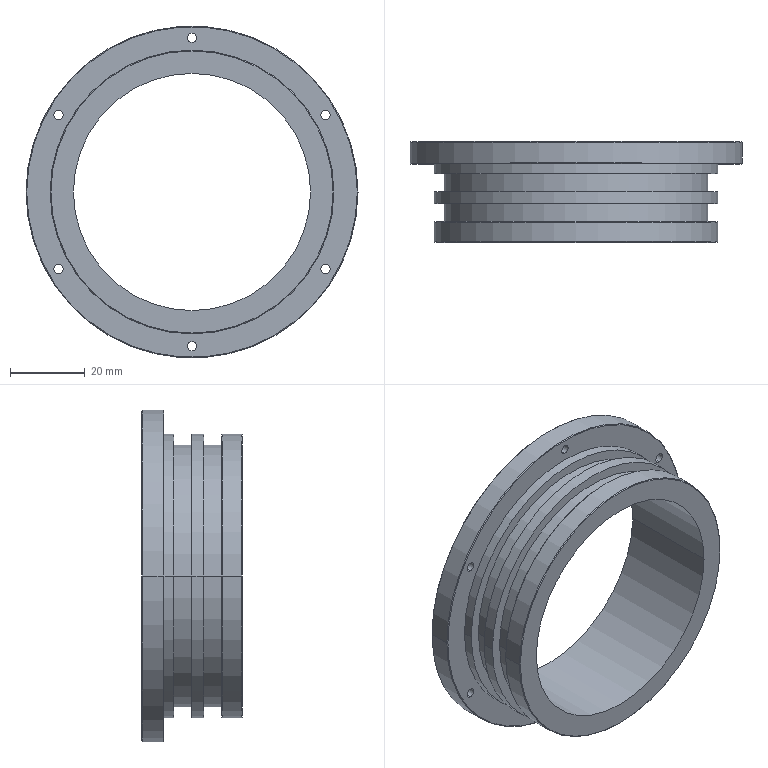Part | SolidWorks | features Chamfer 2, HoleWzd 1, ICE 1, Revolution 1 | 1 solid | 51 faces | box 88.9 x 27 x 88.9 mm | volume 39147 mm3 | cylinder 30 | cone 12 | plane 9 | commonest cylinder face diameters 2.5 x12 75.946 x6 70.561 x4 63.5 x2 70 x2 74.5 x2
STEP:
#1=CARTESIAN_POINT('',(-34.8,27.,0.));
#2=VERTEX_POINT('',#1);
#3=CARTESIAN_POINT('',(34.8,27.,0.));
#4=VERTEX_POINT('',#3);
#5=CARTESIAN_POINT('',(0.,27.,0.));
#6=DIRECTION('',(0.,1.,0.));
#7=DIRECTION('',(-1.,0.,0.));
#8=AXIS2_PLACEMENT_3D('',#5,#6,#7);
#9=CIRCLE('',#8,34.8);
#10=EDGE_CURVE('',#2,#4,#9,.T.);
#11=ORIENTED_EDGE('',*,*,#10,.F.);
#12=CARTESIAN_POINT('',(-35.,26.8,0.));
#13=VERTEX_POINT('',#12);
#14=CARTESIAN_POINT('',(-34.8,27.,0.));
#15=DIRECTION('',(-0.7071,-0.7071,0.));
#16=VECTOR('',#15,1000.);
#17=LINE('',#14,#16);
#18=EDGE_CURVE('',#2,#13,#17,.T.);
#19=ORIENTED_EDGE('',*,*,#18,.T.);
#20=CARTESIAN_POINT('',(35.,26.8,0.));
#21=VERTEX_POINT('',#20);
#22=CARTESIAN_POINT('',(0.,26.8,0.));
#23=DIRECTION('',(0.,-1.,0.));
#24=DIRECTION('',(-1.,0.,0.));
#25=AXIS2_PLACEMENT_3D('',#22,#23,#24);
#26=CIRCLE('',#25,35.);
#27=EDGE_CURVE('',#21,#13,#26,.T.);
#28=ORIENTED_EDGE('',*,*,#27,.F.);
#29=CARTESIAN_POINT('',(34.8,27.,0.));
#30=DIRECTION('',(0.7071,-0.7071,0.));
#31=VECTOR('',#30,1000.);
#32=LINE('',#29,#31);
#33=EDGE_CURVE('',#4,#21,#32,.T.);
#34=ORIENTED_EDGE('',*,*,#33,.F.);
#35=EDGE_LOOP('',(#11,#19,#28,#34));
#36=FACE_OUTER_BOUND('',#35,.T.);
#37=CARTESIAN_POINT('',(0.,27.,0.));
#38=DIRECTION('',(0.,-1.,0.));
#39=DIRECTION('',(1.,0.,0.));
#40=AXIS2_PLACEMENT_3D('',#37,#38,#39);
#41=CONICAL_SURFACE('',#40,34.8,0.7854);
#42=ADVANCED_FACE('',(#36),#41,.T.);
#43=CARTESIAN_POINT('',(37.25,26.8,0.));
#44=VERTEX_POINT('',#43);
#45=CARTESIAN_POINT('',(-37.25,26.8,0.));
#46=VERTEX_POINT('',#45);
#47=CARTESIAN_POINT('',(0.,26.8,0.));
#48=DIRECTION('',(0.,1.,0.));
#49=DIRECTION('',(-1.,0.,0.));
#50=AXIS2_PLACEMENT_3D('',#47,#48,#49);
#51=CIRCLE('',#50,37.25);
#52=EDGE_CURVE('',#44,#46,#51,.T.);
#53=ORIENTED_EDGE('',*,*,#52,.F.);
#54=CARTESIAN_POINT('',(37.45,27.,0.));
#55=VERTEX_POINT('',#54);
#56=CARTESIAN_POINT('',(37.25,26.8,0.));
#57=DIRECTION('',(0.7071,0.7071,0.));
#58=VECTOR('',#57,1000.);
#59=LINE('',#56,#58);
#60=EDGE_CURVE('',#44,#55,#59,.T.);
#61=ORIENTED_EDGE('',*,*,#60,.T.);
#62=CARTESIAN_POINT('',(-37.45,27.,0.));
#63=VERTEX_POINT('',#62);
#64=CARTESIAN_POINT('',(0.,27.,0.));
#65=DIRECTION('',(0.,-1.,0.));
#66=DIRECTION('',(-1.,0.,0.));
#67=AXIS2_PLACEMENT_3D('',#64,#65,#66);
#68=CIRCLE('',#67,37.45);
#69=EDGE_CURVE('',#63,#55,#68,.T.);
#70=ORIENTED_EDGE('',*,*,#69,.F.);
#71=CARTESIAN_POINT('',(-37.25,26.8,0.));
#72=DIRECTION('',(-0.7071,0.7071,0.));
#73=VECTOR('',#72,1000.);
#74=LINE('',#71,#73);
#75=EDGE_CURVE('',#46,#63,#74,.T.);
#76=ORIENTED_EDGE('',*,*,#75,.F.);
#77=EDGE_LOOP('',(#53,#61,#70,#76));
#78=FACE_OUTER_BOUND('',#77,.T.);
#79=CARTESIAN_POINT('',(0.,26.8,0.));
#80=DIRECTION('',(0.,1.,0.));
#81=DIRECTION('',(-1.,0.,0.));
#82=AXIS2_PLACEMENT_3D('',#79,#80,#81);
#83=CONICAL_SURFACE('',#82,37.25,0.7854);
#84=ADVANCED_FACE('',(#78),#83,.F.);
#85=CARTESIAN_POINT('',(-35.,24.,0.));
#86=VERTEX_POINT('',#85);
#87=CARTESIAN_POINT('',(35.,24.,0.));
#88=VERTEX_POINT('',#87);
#89=CARTESIAN_POINT('',(0.,24.,0.));
#90=DIRECTION('',(0.,1.,0.));
#91=DIRECTION('',(-1.,0.,0.));
#92=AXIS2_PLACEMENT_3D('',#89,#90,#91);
#93=CIRCLE('',#92,35.);
#94=EDGE_CURVE('',#86,#88,#93,.T.);
#95=ORIENTED_EDGE('',*,*,#94,.T.);
#96=CARTESIAN_POINT('',(35.,24.,0.));
#97=DIRECTION('',(0.,1.,0.));
#98=VECTOR('',#97,1000.);
#99=LINE('',#96,#98);
#100=EDGE_CURVE('',#88,#21,#99,.T.);
#101=ORIENTED_EDGE('',*,*,#100,.T.);
#102=ORIENTED_EDGE('',*,*,#27,.T.);
#103=CARTESIAN_POINT('',(-35.,24.,0.));
#104=DIRECTION('',(0.,1.,0.));
#105=VECTOR('',#104,1000.);
#106=LINE('',#103,#105);
#107=EDGE_CURVE('',#86,#13,#106,.T.);
#108=ORIENTED_EDGE('',*,*,#107,.F.);
#109=EDGE_LOOP('',(#95,#101,#102,#108));
#110=FACE_OUTER_BOUND('',#109,.T.);
#111=CARTESIAN_POINT('',(0.,24.,0.));
#112=DIRECTION('',(0.,1.,0.));
#113=DIRECTION('',(-1.,0.,0.));
#114=AXIS2_PLACEMENT_3D('',#111,#112,#113);
#115=CYLINDRICAL_SURFACE('',#114,35.);
#116=ADVANCED_FACE('',(#110),#115,.T.);
#117=CARTESIAN_POINT('',(37.25,24.,0.));
#118=VERTEX_POINT('',#117);
#119=CARTESIAN_POINT('',(-37.25,24.,0.));
#120=VERTEX_POINT('',#119);
#121=CARTESIAN_POINT('',(0.,24.,0.));
#122=DIRECTION('',(0.,1.,0.));
#123=DIRECTION('',(-1.,0.,0.));
#124=AXIS2_PLACEMENT_3D('',#121,#122,#123);
#125=CIRCLE('',#124,37.25);
#126=EDGE_CURVE('',#118,#120,#125,.T.);
#127=ORIENTED_EDGE('',*,*,#126,.F.);
#128=CARTESIAN_POINT('',(37.25,24.,0.));
#129=DIRECTION('',(0.,1.,0.));
#130=VECTOR('',#129,1000.);
#131=LINE('',#128,#130);
#132=EDGE_CURVE('',#118,#44,#131,.T.);
#133=ORIENTED_EDGE('',*,*,#132,.T.);
#134=ORIENTED_EDGE('',*,*,#52,.T.);
#135=CARTESIAN_POINT('',(-37.25,24.,0.));
#136=DIRECTION('',(0.,1.,0.));
#137=VECTOR('',#136,1000.);
#138=LINE('',#135,#137);
#139=EDGE_CURVE('',#120,#46,#138,.T.);
#140=ORIENTED_EDGE('',*,*,#139,.F.);
#141=EDGE_LOOP('',(#127,#133,#134,#140));
#142=FACE_OUTER_BOUND('',#141,.T.);
#143=CARTESIAN_POINT('',(0.,24.,0.));
#144=DIRECTION('',(0.,1.,0.));
#145=DIRECTION('',(-1.,0.,0.));
#146=AXIS2_PLACEMENT_3D('',#143,#144,#145);
#147=CYLINDRICAL_SURFACE('',#146,37.25);
#148=ADVANCED_FACE('',(#142),#147,.F.);
#149=CARTESIAN_POINT('',(-35.745,21.,21.888));
#150=VERTEX_POINT('',#149);
#151=CARTESIAN_POINT('',(-35.745,21.,19.388));
#152=VERTEX_POINT('',#151);
#153=CARTESIAN_POINT('',(-35.745,21.,20.638));
#154=DIRECTION('',(0.,-1.,0.));
#155=DIRECTION('',(1.,0.,0.));
#156=AXIS2_PLACEMENT_3D('',#153,#154,#155);
#157=CIRCLE('',#156,1.25);
#158=EDGE_CURVE('',#150,#152,#157,.T.);
#159=ORIENTED_EDGE('',*,*,#158,.T.);
#160=CARTESIAN_POINT('',(-35.745,27.,19.388));
#161=VERTEX_POINT('',#160);
#162=CARTESIAN_POINT('',(-35.745,27.,19.388));
#163=DIRECTION('',(0.,1.,0.));
#164=VECTOR('',#163,1000.);
#165=LINE('',#162,#164);
#166=EDGE_CURVE('',#152,#161,#165,.T.);
#167=ORIENTED_EDGE('',*,*,#166,.T.);
#168=CARTESIAN_POINT('',(-35.745,27.,21.888));
#169=VERTEX_POINT('',#168);
#170=CARTESIAN_POINT('',(-35.745,27.,20.638));
#171=DIRECTION('',(0.,1.,0.));
#172=DIRECTION('',(0.,0.,1.));
#173=AXIS2_PLACEMENT_3D('',#170,#171,#172);
#174=CIRCLE('',#173,1.25);
#175=EDGE_CURVE('',#161,#169,#174,.T.);
#176=ORIENTED_EDGE('',*,*,#175,.T.);
#177=CARTESIAN_POINT('',(-35.745,27.,21.888));
#178=DIRECTION('',(0.,1.,0.));
#179=VECTOR('',#178,1000.);
#180=LINE('',#177,#179);
#181=EDGE_CURVE('',#150,#169,#180,.T.);
#182=ORIENTED_EDGE('',*,*,#181,.F.);
#183=EDGE_LOOP('',(#159,#167,#176,#182));
#184=FACE_OUTER_BOUND('',#183,.T.);
#185=CARTESIAN_POINT('',(-35.745,27.,20.638));
#186=DIRECTION('',(0.,1.,0.));
#187=DIRECTION('',(0.,0.,1.));
#188=AXIS2_PLACEMENT_3D('',#185,#186,#187);
#189=CYLINDRICAL_SURFACE('',#188,1.25);
#190=ADVANCED_FACE('',(#184),#189,.F.);
#191=CARTESIAN_POINT('',(-35.745,21.,-19.388));
#192=VERTEX_POINT('',#191);
#193=CARTESIAN_POINT('',(-35.745,21.,-21.887));
#194=VERTEX_POINT('',#193);
#195=CARTESIAN_POINT('',(-35.745,21.,-20.638));
#196=DIRECTION('',(0.,-1.,0.));
#197=DIRECTION('',(1.,0.,0.));
#198=AXIS2_PLACEMENT_3D('',#195,#196,#197);
#199=CIRCLE('',#198,1.25);
#200=EDGE_CURVE('',#192,#194,#199,.T.);
#201=ORIENTED_EDGE('',*,*,#200,.T.);
#202=CARTESIAN_POINT('',(-35.745,27.,-21.887));
#203=VERTEX_POINT('',#202);
#204=CARTESIAN_POINT('',(-35.745,27.,-21.887));
#205=DIRECTION('',(0.,1.,0.));
#206=VECTOR('',#205,1000.);
#207=LINE('',#204,#206);
#208=EDGE_CURVE('',#194,#203,#207,.T.);
#209=ORIENTED_EDGE('',*,*,#208,.T.);
#210=CARTESIAN_POINT('',(-35.745,27.,-19.388));
#211=VERTEX_POINT('',#210);
#212=CARTESIAN_POINT('',(-35.745,27.,-20.638));
#213=DIRECTION('',(0.,1.,0.));
#214=DIRECTION('',(0.,0.,1.));
#215=AXIS2_PLACEMENT_3D('',#212,#213,#214);
#216=CIRCLE('',#215,1.25);
#217=EDGE_CURVE('',#203,#211,#216,.T.);
#218=ORIENTED_EDGE('',*,*,#217,.T.);
#219=CARTESIAN_POINT('',(-35.745,27.,-19.388));
#220=DIRECTION('',(0.,1.,0.));
#221=VECTOR('',#220,1000.);
#222=LINE('',#219,#221);
#223=EDGE_CURVE('',#192,#211,#222,.T.);
#224=ORIENTED_EDGE('',*,*,#223,.F.);
#225=EDGE_LOOP('',(#201,#209,#218,#224));
#226=FACE_OUTER_BOUND('',#225,.T.);
#227=CARTESIAN_POINT('',(-35.745,27.,-20.638));
#228=DIRECTION('',(0.,1.,0.));
#229=DIRECTION('',(0.,0.,1.));
#230=AXIS2_PLACEMENT_3D('',#227,#228,#229);
#231=CYLINDRICAL_SURFACE('',#230,1.25);
#232=ADVANCED_FACE('',(#226),#231,.F.);
#233=CARTESIAN_POINT('',(0.,21.,-40.025));
#234=VERTEX_POINT('',#233);
#235=CARTESIAN_POINT('',(0.,21.,-42.525));
#236=VERTEX_POINT('',#235);
#237=CARTESIAN_POINT('',(0.,21.,-41.275));
#238=DIRECTION('',(0.,-1.,0.));
#239=DIRECTION('',(1.,0.,0.));
#240=AXIS2_PLACEMENT_3D('',#237,#238,#239);
#241=CIRCLE('',#240,1.25);
#242=EDGE_CURVE('',#234,#236,#241,.T.);
#243=ORIENTED_EDGE('',*,*,#242,.T.);
#244=CARTESIAN_POINT('',(0.,27.,-42.525));
#245=VERTEX_POINT('',#244);
#246=CARTESIAN_POINT('',(0.,27.,-42.525));
#247=DIRECTION('',(0.,1.,0.));
#248=VECTOR('',#247,1000.);
#249=LINE('',#246,#248);
#250=EDGE_CURVE('',#236,#245,#249,.T.);
#251=ORIENTED_EDGE('',*,*,#250,.T.);
#252=CARTESIAN_POINT('',(0.,27.,-40.025));
#253=VERTEX_POINT('',#252);
#254=CARTESIAN_POINT('',(0.,27.,-41.275));
#255=DIRECTION('',(0.,1.,0.));
#256=DIRECTION('',(0.,0.,1.));
#257=AXIS2_PLACEMENT_3D('',#254,#255,#256);
#258=CIRCLE('',#257,1.25);
#259=EDGE_CURVE('',#245,#253,#258,.T.);
#260=ORIENTED_EDGE('',*,*,#259,.T.);
#261=CARTESIAN_POINT('',(0.,27.,-40.025));
#262=DIRECTION('',(0.,1.,0.));
#263=VECTOR('',#262,1000.);
#264=LINE('',#261,#263);
#265=EDGE_CURVE('',#234,#253,#264,.T.);
#266=ORIENTED_EDGE('',*,*,#265,.F.);
#267=EDGE_LOOP('',(#243,#251,#260,#266));
#268=FACE_OUTER_BOUND('',#267,.T.);
#269=CARTESIAN_POINT('',(0.,27.,-41.275));
#270=DIRECTION('',(0.,1.,0.));
#271=DIRECTION('',(0.,0.,1.));
#272=AXIS2_PLACEMENT_3D('',#269,#270,#271);
#273=CYLINDRICAL_SURFACE('',#272,1.25);
#274=ADVANCED_FACE('',(#268),#273,.F.);
#275=CARTESIAN_POINT('',(35.745,21.,-19.388));
#276=VERTEX_POINT('',#275);
#277=CARTESIAN_POINT('',(35.745,21.,-21.888));
#278=VERTEX_POINT('',#277);
#279=CARTESIAN_POINT('',(35.745,21.,-20.638));
#280=DIRECTION('',(0.,-1.,0.));
#281=DIRECTION('',(1.,0.,0.));
#282=AXIS2_PLACEMENT_3D('',#279,#280,#281);
#283=CIRCLE('',#282,1.25);
#284=EDGE_CURVE('',#276,#278,#283,.T.);
#285=ORIENTED_EDGE('',*,*,#284,.T.);
#286=CARTESIAN_POINT('',(35.745,27.,-21.888));
#287=VERTEX_POINT('',#286);
#288=CARTESIAN_POINT('',(35.745,27.,-21.888));
#289=DIRECTION('',(0.,1.,0.));
#290=VECTOR('',#289,1000.);
#291=LINE('',#288,#290);
#292=EDGE_CURVE('',#278,#287,#291,.T.);
#293=ORIENTED_EDGE('',*,*,#292,.T.);
#294=CARTESIAN_POINT('',(35.745,27.,-19.388));
#295=VERTEX_POINT('',#294);
#296=CARTESIAN_POINT('',(35.745,27.,-20.638));
#297=DIRECTION('',(0.,1.,0.));
#298=DIRECTION('',(0.,0.,1.));
#299=AXIS2_PLACEMENT_3D('',#296,#297,#298);
#300=CIRCLE('',#299,1.25);
#301=EDGE_CURVE('',#287,#295,#300,.T.);
#302=ORIENTED_EDGE('',*,*,#301,.T.);
#303=CARTESIAN_POINT('',(35.745,27.,-19.388));
#304=DIRECTION('',(0.,1.,0.));
#305=VECTOR('',#304,1000.);
#306=LINE('',#303,#305);
#307=EDGE_CURVE('',#276,#295,#306,.T.);
#308=ORIENTED_EDGE('',*,*,#307,.F.);
#309=EDGE_LOOP('',(#285,#293,#302,#308));
#310=FACE_OUTER_BOUND('',#309,.T.);
#311=CARTESIAN_POINT('',(35.745,27.,-20.638));
#312=DIRECTION('',(0.,1.,0.));
#313=DIRECTION('',(0.,0.,1.));
#314=AXIS2_PLACEMENT_3D('',#311,#312,#313);
#315=CYLINDRICAL_SURFACE('',#314,1.25);
#316=ADVANCED_FACE('',(#310),#315,.F.);
#317=CARTESIAN_POINT('',(35.745,21.,21.887));
#318=VERTEX_POINT('',#317);
#319=CARTESIAN_POINT('',(35.745,21.,19.388));
#320=VERTEX_POINT('',#319);
#321=CARTESIAN_POINT('',(35.745,21.,20.637));
#322=DIRECTION('',(0.,-1.,0.));
#323=DIRECTION('',(1.,0.,0.));
#324=AXIS2_PLACEMENT_3D('',#321,#322,#323);
#325=CIRCLE('',#324,1.25);
#326=EDGE_CURVE('',#318,#320,#325,.T.);
#327=ORIENTED_EDGE('',*,*,#326,.T.);
#328=CARTESIAN_POINT('',(35.745,27.,19.388));
#329=VERTEX_POINT('',#328);
#330=CARTESIAN_POINT('',(35.745,27.,19.388));
#331=DIRECTION('',(0.,1.,0.));
#332=VECTOR('',#331,1000.);
#333=LINE('',#330,#332);
#334=EDGE_CURVE('',#320,#329,#333,.T.);
#335=ORIENTED_EDGE('',*,*,#334,.T.);
#336=CARTESIAN_POINT('',(35.745,27.,21.887));
#337=VERTEX_POINT('',#336);
#338=CARTESIAN_POINT('',(35.745,27.,20.637));
#339=DIRECTION('',(0.,1.,0.));
#340=DIRECTION('',(0.,0.,1.));
#341=AXIS2_PLACEMENT_3D('',#338,#339,#340);
#342=CIRCLE('',#341,1.25);
#343=EDGE_CURVE('',#329,#337,#342,.T.);
#344=ORIENTED_EDGE('',*,*,#343,.T.);
#345=CARTESIAN_POINT('',(35.745,27.,21.887));
#346=DIRECTION('',(0.,1.,0.));
#347=VECTOR('',#346,1000.);
#348=LINE('',#345,#347);
#349=EDGE_CURVE('',#318,#337,#348,.T.);
#350=ORIENTED_EDGE('',*,*,#349,.F.);
#351=EDGE_LOOP('',(#327,#335,#344,#350));
#352=FACE_OUTER_BOUND('',#351,.T.);
#353=CARTESIAN_POINT('',(35.745,27.,20.637));
#354=DIRECTION('',(0.,1.,0.));
#355=DIRECTION('',(0.,0.,1.));
#356=AXIS2_PLACEMENT_3D('',#353,#354,#355);
#357=CYLINDRICAL_SURFACE('',#356,1.25);
#358=ADVANCED_FACE('',(#352),#357,.F.);
#359=CARTESIAN_POINT('',(0.,21.,42.525));
#360=VERTEX_POINT('',#359);
#361=CARTESIAN_POINT('',(0.,21.,40.025));
#362=VERTEX_POINT('',#361);
#363=CARTESIAN_POINT('',(0.,21.,41.275));
#364=DIRECTION('',(0.,-1.,0.));
#365=DIRECTION('',(1.,0.,0.));
#366=AXIS2_PLACEMENT_3D('',#363,#364,#365);
#367=CIRCLE('',#366,1.25);
#368=EDGE_CURVE('',#360,#362,#367,.T.);
#369=ORIENTED_EDGE('',*,*,#368,.T.);
#370=CARTESIAN_POINT('',(0.,27.,40.025));
#371=VERTEX_POINT('',#370);
#372=CARTESIAN_POINT('',(0.,27.,40.025));
#373=DIRECTION('',(0.,1.,0.));
#374=VECTOR('',#373,1000.);
#375=LINE('',#372,#374);
#376=EDGE_CURVE('',#362,#371,#375,.T.);
#377=ORIENTED_EDGE('',*,*,#376,.T.);
#378=CARTESIAN_POINT('',(0.,27.,42.525));
#379=VERTEX_POINT('',#378);
#380=CARTESIAN_POINT('',(0.,27.,41.275));
#381=DIRECTION('',(0.,1.,0.));
#382=DIRECTION('',(0.,0.,1.));
#383=AXIS2_PLACEMENT_3D('',#380,#381,#382);
#384=CIRCLE('',#383,1.25);
#385=EDGE_CURVE('',#371,#379,#384,.T.);
#386=ORIENTED_EDGE('',*,*,#385,.T.);
#387=CARTESIAN_POINT('',(0.,27.,42.525));
#388=DIRECTION('',(0.,1.,0.));
#389=VECTOR('',#388,1000.);
#390=LINE('',#387,#389);
#391=EDGE_CURVE('',#360,#379,#390,.T.);
#392=ORIENTED_EDGE('',*,*,#391,.F.);
#393=EDGE_LOOP('',(#369,#377,#386,#392));
#394=FACE_OUTER_BOUND('',#393,.T.);
#395=CARTESIAN_POINT('',(0.,27.,41.275));
#396=DIRECTION('',(0.,1.,0.));
#397=DIRECTION('',(0.,0.,1.));
#398=AXIS2_PLACEMENT_3D('',#395,#396,#397);
#399=CYLINDRICAL_SURFACE('',#398,1.25);
#400=ADVANCED_FACE('',(#394),#399,.F.);
#401=CARTESIAN_POINT('',(44.25,21.,0.));
#402=VERTEX_POINT('',#401);
#403=CARTESIAN_POINT('',(-44.25,21.,0.));
#404=VERTEX_POINT('',#403);
#405=CARTESIAN_POINT('',(0.,21.,0.));
#406=DIRECTION('',(0.,-1.,0.));
#407=DIRECTION('',(1.,0.,0.));
#408=AXIS2_PLACEMENT_3D('',#405,#406,#407);
#409=CIRCLE('',#408,44.25);
#410=EDGE_CURVE('',#402,#404,#409,.T.);
#411=ORIENTED_EDGE('',*,*,#410,.F.);
#412=CARTESIAN_POINT('',(44.45,21.2,0.));
#413=VERTEX_POINT('',#412);
#414=CARTESIAN_POINT('',(44.45,21.2,0.));
#415=DIRECTION('',(0.7071,0.7071,0.));
#416=VECTOR('',#415,1000.);
#417=LINE('',#414,#416);
#418=EDGE_CURVE('',#402,#413,#417,.T.);
#419=ORIENTED_EDGE('',*,*,#418,.T.);
#420=CARTESIAN_POINT('',(-44.45,21.2,0.));
#421=VERTEX_POINT('',#420);
#422=CARTESIAN_POINT('',(0.,21.2,0.));
#423=DIRECTION('',(0.,1.,0.));
#424=DIRECTION('',(1.,0.,0.));
#425=AXIS2_PLACEMENT_3D('',#422,#423,#424);
#426=CIRCLE('',#425,44.45);
#427=EDGE_CURVE('',#421,#413,#426,.T.);
#428=ORIENTED_EDGE('',*,*,#427,.F.);
#429=CARTESIAN_POINT('',(-44.45,21.2,0.));
#430=DIRECTION('',(-0.7071,0.7071,0.));
#431=VECTOR('',#430,1000.);
#432=LINE('',#429,#431);
#433=EDGE_CURVE('',#404,#421,#432,.T.);
#434=ORIENTED_EDGE('',*,*,#433,.F.);
#435=EDGE_LOOP('',(#411,#419,#428,#434));
#436=FACE_OUTER_BOUND('',#435,.T.);
#437=CARTESIAN_POINT('',(0.,21.2,0.));
#438=DIRECTION('',(0.,1.,0.));
#439=DIRECTION('',(-1.,0.,0.));
#440=AXIS2_PLACEMENT_3D('',#437,#438,#439);
#441=CONICAL_SURFACE('',#440,44.45,0.7854);
#442=ADVANCED_FACE('',(#436),#441,.T.);
#443=CARTESIAN_POINT('',(-44.25,27.,0.));
#444=VERTEX_POINT('',#443);
#445=CARTESIAN_POINT('',(44.25,27.,0.));
#446=VERTEX_POINT('',#445);
#447=CARTESIAN_POINT('',(0.,27.,0.));
#448=DIRECTION('',(0.,1.,0.));
#449=DIRECTION('',(-1.,0.,0.));
#450=AXIS2_PLACEMENT_3D('',#447,#448,#449);
#451=CIRCLE('',#450,44.25);
#452=EDGE_CURVE('',#444,#446,#451,.T.);
#453=ORIENTED_EDGE('',*,*,#452,.F.);
#454=CARTESIAN_POINT('',(-44.45,26.8,0.));
#455=VERTEX_POINT('',#454);
#456=CARTESIAN_POINT('',(-44.25,27.,0.));
#457=DIRECTION('',(-0.7071,-0.7071,0.));
#458=VECTOR('',#457,1000.);
#459=LINE('',#456,#458);
#460=EDGE_CURVE('',#444,#455,#459,.T.);
#461=ORIENTED_EDGE('',*,*,#460,.T.);
#462=CARTESIAN_POINT('',(44.45,26.8,0.));
#463=VERTEX_POINT('',#462);
#464=CARTESIAN_POINT('',(0.,26.8,0.));
#465=DIRECTION('',(0.,-1.,0.));
#466=DIRECTION('',(-1.,0.,0.));
#467=AXIS2_PLACEMENT_3D('',#464,#465,#466);
#468=CIRCLE('',#467,44.45);
#469=EDGE_CURVE('',#463,#455,#468,.T.);
#470=ORIENTED_EDGE('',*,*,#469,.F.);
#471=CARTESIAN_POINT('',(44.25,27.,0.));
#472=DIRECTION('',(0.7071,-0.7071,0.));
#473=VECTOR('',#472,1000.);
#474=LINE('',#471,#473);
#475=EDGE_CURVE('',#446,#463,#474,.T.);
#476=ORIENTED_EDGE('',*,*,#475,.F.);
#477=EDGE_LOOP('',(#453,#461,#470,#476));
#478=FACE_OUTER_BOUND('',#477,.T.);
#479=CARTESIAN_POINT('',(0.,27.,0.));
#480=DIRECTION('',(0.,-1.,0.));
#481=DIRECTION('',(1.,0.,0.));
#482=AXIS2_PLACEMENT_3D('',#479,#480,#481);
#483=CONICAL_SURFACE('',#482,44.25,0.7854);
#484=ADVANCED_FACE('',(#478),#483,.T.);
#485=CARTESIAN_POINT('',(37.773,0.,0.));
#486=VERTEX_POINT('',#485);
#487=CARTESIAN_POINT('',(-37.773,0.,0.));
#488=VERTEX_POINT('',#487);
#489=CARTESIAN_POINT('',(0.,0.,0.));
#490=DIRECTION('',(0.,-1.,0.));
#491=DIRECTION('',(1.,0.,0.));
#492=AXIS2_PLACEMENT_3D('',#489,#490,#491);
#493=CIRCLE('',#492,37.773);
#494=EDGE_CURVE('',#486,#488,#493,.T.);
#495=ORIENTED_EDGE('',*,*,#494,.F.);
#496=CARTESIAN_POINT('',(37.973,0.2,0.));
#497=VERTEX_POINT('',#496);
#498=CARTESIAN_POINT('',(37.973,0.2,0.));
#499=DIRECTION('',(0.7071,0.7071,0.));
#500=VECTOR('',#499,1000.);
#501=LINE('',#498,#500);
#502=EDGE_CURVE('',#486,#497,#501,.T.);
#503=ORIENTED_EDGE('',*,*,#502,.T.);
#504=CARTESIAN_POINT('',(-37.973,0.2,0.));
#505=VERTEX_POINT('',#504);
#506=CARTESIAN_POINT('',(0.,0.2,0.));
#507=DIRECTION('',(0.,1.,0.));
#508=DIRECTION('',(1.,0.,0.));
#509=AXIS2_PLACEMENT_3D('',#506,#507,#508);
#510=CIRCLE('',#509,37.973);
#511=EDGE_CURVE('',#505,#497,#510,.T.);
#512=ORIENTED_EDGE('',*,*,#511,.F.);
#513=CARTESIAN_POINT('',(-37.973,0.2,0.));
#514=DIRECTION('',(-0.7071,0.7071,0.));
#515=VECTOR('',#514,1000.);
#516=LINE('',#513,#515);
#517=EDGE_CURVE('',#488,#505,#516,.T.);
#518=ORIENTED_EDGE('',*,*,#517,.F.);
#519=EDGE_LOOP('',(#495,#503,#512,#518));
#520=FACE_OUTER_BOUND('',#519,.T.);
#521=CARTESIAN_POINT('',(0.,0.2,0.));
#522=DIRECTION('',(0.,1.,0.));
#523=DIRECTION('',(-1.,0.,0.));
#524=AXIS2_PLACEMENT_3D('',#521,#522,#523);
#525=CONICAL_SURFACE('',#524,37.973,0.7854);
#526=ADVANCED_FACE('',(#520),#525,.T.);
#527=CARTESIAN_POINT('',(-37.773,5.587,0.));
#528=VERTEX_POINT('',#527);
#529=CARTESIAN_POINT('',(37.773,5.587,0.));
#530=VERTEX_POINT('',#529);
#531=CARTESIAN_POINT('',(0.,5.587,0.));
#532=DIRECTION('',(0.,1.,0.));
#533=DIRECTION('',(-1.,0.,0.));
#534=AXIS2_PLACEMENT_3D('',#531,#532,#533);
#535=CIRCLE('',#534,37.773);
#536=EDGE_CURVE('',#528,#530,#535,.T.);
#537=ORIENTED_EDGE('',*,*,#536,.F.);
#538=CARTESIAN_POINT('',(-37.973,5.387,0.));
#539=VERTEX_POINT('',#538);
#540=CARTESIAN_POINT('',(-37.773,5.587,0.));
#541=DIRECTION('',(-0.7071,-0.7071,0.));
#542=VECTOR('',#541,1000.);
#543=LINE('',#540,#542);
#544=EDGE_CURVE('',#528,#539,#543,.T.);
#545=ORIENTED_EDGE('',*,*,#544,.T.);
#546=CARTESIAN_POINT('',(37.973,5.387,0.));
#547=VERTEX_POINT('',#546);
#548=CARTESIAN_POINT('',(0.,5.387,0.));
#549=DIRECTION('',(0.,-1.,0.));
#550=DIRECTION('',(-1.,0.,0.));
#551=AXIS2_PLACEMENT_3D('',#548,#549,#550);
#552=CIRCLE('',#551,37.973);
#553=EDGE_CURVE('',#547,#539,#552,.T.);
#554=ORIENTED_EDGE('',*,*,#553,.F.);
#555=CARTESIAN_POINT('',(37.773,5.587,0.));
#556=DIRECTION('',(0.7071,-0.7071,0.));
#557=VECTOR('',#556,1000.);
#558=LINE('',#555,#557);
#559=EDGE_CURVE('',#530,#547,#558,.T.);
#560=ORIENTED_EDGE('',*,*,#559,.F.);
#561=EDGE_LOOP('',(#537,#545,#554,#560));
#562=FACE_OUTER_BOUND('',#561,.T.);
#563=CARTESIAN_POINT('',(0.,5.587,0.));
#564=DIRECTION('',(0.,-1.,0.));
#565=DIRECTION('',(1.,0.,0.));
#566=AXIS2_PLACEMENT_3D('',#563,#564,#565);
#567=CONICAL_SURFACE('',#566,37.773,0.7854);
#568=ADVANCED_FACE('',(#562),#567,.T.);
#569=ORIENTED_EDGE('',*,*,#427,.T.);
#570=CARTESIAN_POINT('',(44.45,27.,0.));
#571=DIRECTION('',(0.,1.,0.));
#572=VECTOR('',#571,1000.);
#573=LINE('',#570,#572);
#574=EDGE_CURVE('',#413,#463,#573,.T.);
#575=ORIENTED_EDGE('',*,*,#574,.T.);
#576=ORIENTED_EDGE('',*,*,#469,.T.);
#577=CARTESIAN_POINT('',(-44.45,27.,0.));
#578=DIRECTION('',(0.,1.,0.));
#579=VECTOR('',#578,1000.);
#580=LINE('',#577,#579);
#581=EDGE_CURVE('',#421,#455,#580,.T.);
#582=ORIENTED_EDGE('',*,*,#581,.F.);
#583=EDGE_LOOP('',(#569,#575,#576,#582));
#584=FACE_OUTER_BOUND('',#583,.T.);
#585=CARTESIAN_POINT('',(0.,27.,0.));
#586=DIRECTION('',(0.,1.,0.));
#587=DIRECTION('',(-1.,0.,0.));
#588=AXIS2_PLACEMENT_3D('',#585,#586,#587);
#589=CYLINDRICAL_SURFACE('',#588,44.45);
#590=ADVANCED_FACE('',(#584),#589,.T.);
#591=CARTESIAN_POINT('',(-37.973,18.413,0.));
#592=VERTEX_POINT('',#591);
#593=CARTESIAN_POINT('',(37.973,18.413,0.));
#594=VERTEX_POINT('',#593);
#595=CARTESIAN_POINT('',(0.,18.413,0.));
#596=DIRECTION('',(0.,1.,0.));
#597=DIRECTION('',(-1.,0.,0.));
#598=AXIS2_PLACEMENT_3D('',#595,#596,#597);
#599=CIRCLE('',#598,37.973);
#600=EDGE_CURVE('',#592,#594,#599,.T.);
#601=ORIENTED_EDGE('',*,*,#600,.T.);
#602=CARTESIAN_POINT('',(37.973,21.,0.));
#603=VERTEX_POINT('',#602);
#604=CARTESIAN_POINT('',(37.973,27.,0.));
#605=DIRECTION('',(0.,1.,0.));
#606=VECTOR('',#605,1000.);
#607=LINE('',#604,#606);
#608=EDGE_CURVE('',#594,#603,#607,.T.);
#609=ORIENTED_EDGE('',*,*,#608,.T.);
#610=CARTESIAN_POINT('',(-37.973,21.,0.));
#611=VERTEX_POINT('',#610);
#612=CARTESIAN_POINT('',(0.,21.,0.));
#613=DIRECTION('',(0.,1.,0.));
#614=DIRECTION('',(-1.,0.,0.));
#615=AXIS2_PLACEMENT_3D('',#612,#613,#614);
#616=CIRCLE('',#615,37.973);
#617=EDGE_CURVE('',#611,#603,#616,.T.);
#618=ORIENTED_EDGE('',*,*,#617,.F.);
#619=CARTESIAN_POINT('',(-37.973,27.,0.));
#620=DIRECTION('',(0.,1.,0.));
#621=VECTOR('',#620,1000.);
#622=LINE('',#619,#621);
#623=EDGE_CURVE('',#592,#611,#622,.T.);
#624=ORIENTED_EDGE('',*,*,#623,.F.);
#625=EDGE_LOOP('',(#601,#609,#618,#624));
#626=FACE_OUTER_BOUND('',#625,.T.);
#627=CARTESIAN_POINT('',(0.,27.,0.));
#628=DIRECTION('',(0.,1.,0.));
#629=DIRECTION('',(-1.,0.,0.));
#630=AXIS2_PLACEMENT_3D('',#627,#628,#629);
#631=CYLINDRICAL_SURFACE('',#630,37.973);
#632=ADVANCED_FACE('',(#626),#631,.T.);
#633=CARTESIAN_POINT('',(-35.281,13.587,0.));
#634=VERTEX_POINT('',#633);
#635=CARTESIAN_POINT('',(35.281,13.587,0.));
#636=VERTEX_POINT('',#635);
#637=CARTESIAN_POINT('',(0.,13.587,0.));
#638=DIRECTION('',(0.,1.,0.));
#639=DIRECTION('',(-1.,0.,0.));
#640=AXIS2_PLACEMENT_3D('',#637,#638,#639);
#641=CIRCLE('',#640,35.281);
#642=EDGE_CURVE('',#634,#636,#641,.T.);
#643=ORIENTED_EDGE('',*,*,#642,.T.);
#644=CARTESIAN_POINT('',(35.281,18.413,0.));
#645=VERTEX_POINT('',#644);
#646=CARTESIAN_POINT('',(35.281,27.,0.));
#647=DIRECTION('',(0.,1.,0.));
#648=VECTOR('',#647,1000.);
#649=LINE('',#646,#648);
#650=EDGE_CURVE('',#636,#645,#649,.T.);
#651=ORIENTED_EDGE('',*,*,#650,.T.);
#652=CARTESIAN_POINT('',(-35.281,18.413,0.));
#653=VERTEX_POINT('',#652);
#654=CARTESIAN_POINT('',(0.,18.413,0.));
#655=DIRECTION('',(0.,1.,0.));
#656=DIRECTION('',(-1.,0.,0.));
#657=AXIS2_PLACEMENT_3D('',#654,#655,#656);
#658=CIRCLE('',#657,35.281);
#659=EDGE_CURVE('',#653,#645,#658,.T.);
#660=ORIENTED_EDGE('',*,*,#659,.F.);
#661=CARTESIAN_POINT('',(-35.281,27.,0.));
#662=DIRECTION('',(0.,1.,0.));
#663=VECTOR('',#662,1000.);
#664=LINE('',#661,#663);
#665=EDGE_CURVE('',#634,#653,#664,.T.);
#666=ORIENTED_EDGE('',*,*,#665,.F.);
#667=EDGE_LOOP('',(#643,#651,#660,#666));
#668=FACE_OUTER_BOUND('',#667,.T.);
#669=CARTESIAN_POINT('',(0.,27.,0.));
#670=DIRECTION('',(0.,1.,0.));
#671=DIRECTION('',(-1.,0.,0.));
#672=AXIS2_PLACEMENT_3D('',#669,#670,#671);
#673=CYLINDRICAL_SURFACE('',#672,35.281);
#674=ADVANCED_FACE('',(#668),#673,.T.);
#675=CARTESIAN_POINT('',(-37.973,10.413,0.));
#676=VERTEX_POINT('',#675);
#677=CARTESIAN_POINT('',(37.973,10.413,0.));
#678=VERTEX_POINT('',#677);
#679=CARTESIAN_POINT('',(0.,10.413,0.));
#680=DIRECTION('',(0.,1.,0.));
#681=DIRECTION('',(-1.,0.,0.));
#682=AXIS2_PLACEMENT_3D('',#679,#680,#681);
#683=CIRCLE('',#682,37.973);
#684=EDGE_CURVE('',#676,#678,#683,.T.);
#685=ORIENTED_EDGE('',*,*,#684,.T.);
#686=CARTESIAN_POINT('',(37.973,13.587,0.));
#687=VERTEX_POINT('',#686);
#688=CARTESIAN_POINT('',(37.973,27.,0.));
#689=DIRECTION('',(0.,1.,0.));
#690=VECTOR('',#689,1000.);
#691=LINE('',#688,#690);
#692=EDGE_CURVE('',#678,#687,#691,.T.);
#693=ORIENTED_EDGE('',*,*,#692,.T.);
#694=CARTESIAN_POINT('',(-37.973,13.587,0.));
#695=VERTEX_POINT('',#694);
#696=CARTESIAN_POINT('',(0.,13.587,0.));
#697=DIRECTION('',(0.,1.,0.));
#698=DIRECTION('',(-1.,0.,0.));
#699=AXIS2_PLACEMENT_3D('',#696,#697,#698);
#700=CIRCLE('',#699,37.973);
#701=EDGE_CURVE('',#695,#687,#700,.T.);
#702=ORIENTED_EDGE('',*,*,#701,.F.);
#703=CARTESIAN_POINT('',(-37.973,27.,0.));
#704=DIRECTION('',(0.,1.,0.));
#705=VECTOR('',#704,1000.);
#706=LINE('',#703,#705);
#707=EDGE_CURVE('',#676,#695,#706,.T.);
#708=ORIENTED_EDGE('',*,*,#707,.F.);
#709=EDGE_LOOP('',(#685,#693,#702,#708));
#710=FACE_OUTER_BOUND('',#709,.T.);
#711=CARTESIAN_POINT('',(0.,27.,0.));
#712=DIRECTION('',(0.,1.,0.));
#713=DIRECTION('',(-1.,0.,0.));
#714=AXIS2_PLACEMENT_3D('',#711,#712,#713);
#715=CYLINDRICAL_SURFACE('',#714,37.973);
#716=ADVANCED_FACE('',(#710),#715,.T.);
#717=CARTESIAN_POINT('',(-35.281,5.587,0.));
#718=VERTEX_POINT('',#717);
#719=CARTESIAN_POINT('',(35.281,5.587,0.));
#720=VERTEX_POINT('',#719);
#721=CARTESIAN_POINT('',(0.,5.587,0.));
#722=DIRECTION('',(0.,1.,0.));
#723=DIRECTION('',(-1.,0.,0.));
#724=AXIS2_PLACEMENT_3D('',#721,#722,#723);
#725=CIRCLE('',#724,35.281);
#726=EDGE_CURVE('',#718,#720,#725,.T.);
#727=ORIENTED_EDGE('',*,*,#726,.T.);
#728=CARTESIAN_POINT('',(35.281,10.413,0.));
#729=VERTEX_POINT('',#728);
#730=CARTESIAN_POINT('',(35.281,27.,0.));
#731=DIRECTION('',(0.,1.,0.));
#732=VECTOR('',#731,1000.);
#733=LINE('',#730,#732);
#734=EDGE_CURVE('',#720,#729,#733,.T.);
#735=ORIENTED_EDGE('',*,*,#734,.T.);
#736=CARTESIAN_POINT('',(-35.281,10.413,0.));
#737=VERTEX_POINT('',#736);
#738=CARTESIAN_POINT('',(0.,10.413,0.));
#739=DIRECTION('',(0.,1.,0.));
#740=DIRECTION('',(-1.,0.,0.));
#741=AXIS2_PLACEMENT_3D('',#738,#739,#740);
#742=CIRCLE('',#741,35.281);
#743=EDGE_CURVE('',#737,#729,#742,.T.);
#744=ORIENTED_EDGE('',*,*,#743,.F.);
#745=CARTESIAN_POINT('',(-35.281,27.,0.));
#746=DIRECTION('',(0.,1.,0.));
#747=VECTOR('',#746,1000.);
#748=LINE('',#745,#747);
#749=EDGE_CURVE('',#718,#737,#748,.T.);
#750=ORIENTED_EDGE('',*,*,#749,.F.);
#751=EDGE_LOOP('',(#727,#735,#744,#750));
#752=FACE_OUTER_BOUND('',#751,.T.);
#753=CARTESIAN_POINT('',(0.,27.,0.));
#754=DIRECTION('',(0.,1.,0.));
#755=DIRECTION('',(-1.,0.,0.));
#756=AXIS2_PLACEMENT_3D('',#753,#754,#755);
#757=CYLINDRICAL_SURFACE('',#756,35.281);
#758=ADVANCED_FACE('',(#752),#757,.T.);
#759=ORIENTED_EDGE('',*,*,#511,.T.);
#760=CARTESIAN_POINT('',(37.973,27.,0.));
#761=DIRECTION('',(0.,1.,0.));
#762=VECTOR('',#761,1000.);
#763=LINE('',#760,#762);
#764=EDGE_CURVE('',#497,#547,#763,.T.);
#765=ORIENTED_EDGE('',*,*,#764,.T.);
#766=ORIENTED_EDGE('',*,*,#553,.T.);
#767=CARTESIAN_POINT('',(-37.973,27.,0.));
#768=DIRECTION('',(0.,1.,0.));
#769=VECTOR('',#768,1000.);
#770=LINE('',#767,#769);
#771=EDGE_CURVE('',#505,#539,#770,.T.);
#772=ORIENTED_EDGE('',*,*,#771,.F.);
#773=EDGE_LOOP('',(#759,#765,#766,#772));
#774=FACE_OUTER_BOUND('',#773,.T.);
#775=CARTESIAN_POINT('',(0.,27.,0.));
#776=DIRECTION('',(0.,1.,0.));
#777=DIRECTION('',(-1.,0.,0.));
#778=AXIS2_PLACEMENT_3D('',#775,#776,#777);
#779=CYLINDRICAL_SURFACE('',#778,37.973);
#780=ADVANCED_FACE('',(#774),#779,.T.);
#781=CARTESIAN_POINT('',(31.75,0.,0.));
#782=VERTEX_POINT('',#781);
#783=CARTESIAN_POINT('',(-31.75,0.,0.));
#784=VERTEX_POINT('',#783);
#785=CARTESIAN_POINT('',(0.,0.,0.));
#786=DIRECTION('',(0.,1.,0.));
#787=DIRECTION('',(-1.,0.,0.));
#788=AXIS2_PLACEMENT_3D('',#785,#786,#787);
#789=CIRCLE('',#788,31.75);
#790=EDGE_CURVE('',#782,#784,#789,.T.);
#791=ORIENTED_EDGE('',*,*,#790,.F.);
#792=CARTESIAN_POINT('',(31.75,27.,0.));
#793=VERTEX_POINT('',#792);
#794=CARTESIAN_POINT('',(31.75,27.,0.));
#795=DIRECTION('',(0.,1.,0.));
#796=VECTOR('',#795,1000.);
#797=LINE('',#794,#796);
#798=EDGE_CURVE('',#782,#793,#797,.T.);
#799=ORIENTED_EDGE('',*,*,#798,.T.);
#800=CARTESIAN_POINT('',(-31.75,27.,0.));
#801=VERTEX_POINT('',#800);
#802=CARTESIAN_POINT('',(0.,27.,0.));
#803=DIRECTION('',(0.,1.,0.));
#804=DIRECTION('',(-1.,0.,0.));
#805=AXIS2_PLACEMENT_3D('',#802,#803,#804);
#806=CIRCLE('',#805,31.75);
#807=EDGE_CURVE('',#793,#801,#806,.T.);
#808=ORIENTED_EDGE('',*,*,#807,.T.);
#809=CARTESIAN_POINT('',(-31.75,27.,0.));
#810=DIRECTION('',(0.,1.,0.));
#811=VECTOR('',#810,1000.);
#812=LINE('',#809,#811);
#813=EDGE_CURVE('',#784,#801,#812,.T.);
#814=ORIENTED_EDGE('',*,*,#813,.F.);
#815=EDGE_LOOP('',(#791,#799,#808,#814));
#816=FACE_OUTER_BOUND('',#815,.T.);
#817=CARTESIAN_POINT('',(0.,27.,0.));
#818=DIRECTION('',(0.,1.,0.));
#819=DIRECTION('',(-1.,0.,0.));
#820=AXIS2_PLACEMENT_3D('',#817,#818,#819);
#821=CYLINDRICAL_SURFACE('',#820,31.75);
#822=ADVANCED_FACE('',(#816),#821,.F.);
#823=CARTESIAN_POINT('',(0.,27.,0.));
#824=DIRECTION('',(0.,1.,0.));
#825=DIRECTION('',(-1.,0.,0.));
#826=AXIS2_PLACEMENT_3D('',#823,#824,#825);
#827=CIRCLE('',#826,34.8);
#828=EDGE_CURVE('',#4,#2,#827,.T.);
#829=ORIENTED_EDGE('',*,*,#828,.T.);
#830=ORIENTED_EDGE('',*,*,#10,.T.);
#831=EDGE_LOOP('',(#829,#830));
#832=FACE_OUTER_BOUND('',#831,.T.);
#833=CARTESIAN_POINT('',(0.,27.,0.));
#834=DIRECTION('',(0.,1.,0.));
#835=DIRECTION('',(-1.,0.,0.));
#836=AXIS2_PLACEMENT_3D('',#833,#834,#835);
#837=CIRCLE('',#836,31.75);
#838=EDGE_CURVE('',#801,#793,#837,.T.);
#839=ORIENTED_EDGE('',*,*,#838,.F.);
#840=ORIENTED_EDGE('',*,*,#807,.F.);
#841=EDGE_LOOP('',(#839,#840));
#842=FACE_BOUND('',#841,.T.);
#843=CARTESIAN_POINT('',(-44.45,27.,0.));
#844=DIRECTION('',(0.,1.,0.));
#845=DIRECTION('',(-1.,0.,0.));
#846=AXIS2_PLACEMENT_3D('',#843,#844,#845);
#847=PLANE('',#846);
#848=ADVANCED_FACE('',(#832,#842),#847,.T.);
#849=ORIENTED_EDGE('',*,*,#69,.T.);
#850=CARTESIAN_POINT('',(0.,27.,0.));
#851=DIRECTION('',(0.,-1.,0.));
#852=DIRECTION('',(-1.,0.,0.));
#853=AXIS2_PLACEMENT_3D('',#850,#851,#852);
#854=CIRCLE('',#853,37.45);
#855=EDGE_CURVE('',#55,#63,#854,.T.);
#856=ORIENTED_EDGE('',*,*,#855,.T.);
#857=EDGE_LOOP('',(#849,#856));
#858=FACE_BOUND('',#857,.T.);
#859=CARTESIAN_POINT('',(-35.745,27.,20.638));
#860=DIRECTION('',(0.,1.,0.));
#861=DIRECTION('',(0.,0.,1.));
#862=AXIS2_PLACEMENT_3D('',#859,#860,#861);
#863=CIRCLE('',#862,1.25);
#864=EDGE_CURVE('',#169,#161,#863,.T.);
#865=ORIENTED_EDGE('',*,*,#864,.F.);
#866=ORIENTED_EDGE('',*,*,#175,.F.);
#867=EDGE_LOOP('',(#865,#866));
#868=FACE_BOUND('',#867,.T.);
#869=CARTESIAN_POINT('',(-35.745,27.,-20.638));
#870=DIRECTION('',(0.,1.,0.));
#871=DIRECTION('',(0.,0.,1.));
#872=AXIS2_PLACEMENT_3D('',#869,#870,#871);
#873=CIRCLE('',#872,1.25);
#874=EDGE_CURVE('',#211,#203,#873,.T.);
#875=ORIENTED_EDGE('',*,*,#874,.F.);
#876=ORIENTED_EDGE('',*,*,#217,.F.);
#877=EDGE_LOOP('',(#875,#876));
#878=FACE_BOUND('',#877,.T.);
#879=CARTESIAN_POINT('',(0.,27.,-41.275));
#880=DIRECTION('',(0.,1.,0.));
#881=DIRECTION('',(0.,0.,1.));
#882=AXIS2_PLACEMENT_3D('',#879,#880,#881);
#883=CIRCLE('',#882,1.25);
#884=EDGE_CURVE('',#253,#245,#883,.T.);
#885=ORIENTED_EDGE('',*,*,#884,.F.);
#886=ORIENTED_EDGE('',*,*,#259,.F.);
#887=EDGE_LOOP('',(#885,#886));
#888=FACE_BOUND('',#887,.T.);
#889=CARTESIAN_POINT('',(35.745,27.,-20.638));
#890=DIRECTION('',(0.,1.,0.));
#891=DIRECTION('',(0.,0.,1.));
#892=AXIS2_PLACEMENT_3D('',#889,#890,#891);
#893=CIRCLE('',#892,1.25);
#894=EDGE_CURVE('',#295,#287,#893,.T.);
#895=ORIENTED_EDGE('',*,*,#894,.F.);
#896=ORIENTED_EDGE('',*,*,#301,.F.);
#897=EDGE_LOOP('',(#895,#896));
#898=FACE_BOUND('',#897,.T.);
#899=CARTESIAN_POINT('',(35.745,27.,20.637));
#900=DIRECTION('',(0.,1.,0.));
#901=DIRECTION('',(0.,0.,1.));
#902=AXIS2_PLACEMENT_3D('',#899,#900,#901);
#903=CIRCLE('',#902,1.25);
#904=EDGE_CURVE('',#337,#329,#903,.T.);
#905=ORIENTED_EDGE('',*,*,#904,.F.);
#906=ORIENTED_EDGE('',*,*,#343,.F.);
#907=EDGE_LOOP('',(#905,#906));
#908=FACE_BOUND('',#907,.T.);
#909=CARTESIAN_POINT('',(0.,27.,41.275));
#910=DIRECTION('',(0.,1.,0.));
#911=DIRECTION('',(0.,0.,1.));
#912=AXIS2_PLACEMENT_3D('',#909,#910,#911);
#913=CIRCLE('',#912,1.25);
#914=EDGE_CURVE('',#379,#371,#913,.T.);
#915=ORIENTED_EDGE('',*,*,#914,.F.);
#916=ORIENTED_EDGE('',*,*,#385,.F.);
#917=EDGE_LOOP('',(#915,#916));
#918=FACE_BOUND('',#917,.T.);
#919=CARTESIAN_POINT('',(0.,27.,0.));
#920=DIRECTION('',(0.,1.,0.));
#921=DIRECTION('',(-1.,0.,0.));
#922=AXIS2_PLACEMENT_3D('',#919,#920,#921);
#923=CIRCLE('',#922,44.25);
#924=EDGE_CURVE('',#446,#444,#923,.T.);
#925=ORIENTED_EDGE('',*,*,#924,.T.);
#926=ORIENTED_EDGE('',*,*,#452,.T.);
#927=EDGE_LOOP('',(#925,#926));
#928=FACE_OUTER_BOUND('',#927,.T.);
#929=CARTESIAN_POINT('',(-44.45,27.,0.));
#930=DIRECTION('',(0.,1.,0.));
#931=DIRECTION('',(-1.,0.,0.));
#932=AXIS2_PLACEMENT_3D('',#929,#930,#931);
#933=PLANE('',#932);
#934=ADVANCED_FACE('',(#858,#868,#878,#888,#898,#908,#918,#928),#933,.T.);
#935=ORIENTED_EDGE('',*,*,#798,.F.);
#936=CARTESIAN_POINT('',(0.,0.,0.));
#937=DIRECTION('',(0.,1.,0.));
#938=DIRECTION('',(-1.,0.,0.));
#939=AXIS2_PLACEMENT_3D('',#936,#937,#938);
#940=CIRCLE('',#939,31.75);
#941=EDGE_CURVE('',#784,#782,#940,.T.);
#942=ORIENTED_EDGE('',*,*,#941,.F.);
#943=ORIENTED_EDGE('',*,*,#813,.T.);
#944=ORIENTED_EDGE('',*,*,#838,.T.);
#945=EDGE_LOOP('',(#935,#942,#943,#944));
#946=FACE_OUTER_BOUND('',#945,.T.);
#947=CARTESIAN_POINT('',(0.,27.,0.));
#948=DIRECTION('',(0.,1.,0.));
#949=DIRECTION('',(-1.,0.,0.));
#950=AXIS2_PLACEMENT_3D('',#947,#948,#949);
#951=CYLINDRICAL_SURFACE('',#950,31.75);
#952=ADVANCED_FACE('',(#946),#951,.F.);
#953=CARTESIAN_POINT('',(0.,0.,0.));
#954=DIRECTION('',(0.,-1.,0.));
#955=DIRECTION('',(1.,0.,0.));
#956=AXIS2_PLACEMENT_3D('',#953,#954,#955);
#957=CIRCLE('',#956,37.773);
#958=EDGE_CURVE('',#488,#486,#957,.T.);
#959=ORIENTED_EDGE('',*,*,#958,.T.);
#960=ORIENTED_EDGE('',*,*,#494,.T.);
#961=EDGE_LOOP('',(#959,#960));
#962=FACE_OUTER_BOUND('',#961,.T.);
#963=ORIENTED_EDGE('',*,*,#941,.T.);
#964=ORIENTED_EDGE('',*,*,#790,.T.);
#965=EDGE_LOOP('',(#963,#964));
#966=FACE_BOUND('',#965,.T.);
#967=CARTESIAN_POINT('',(-31.75,0.,0.));
#968=DIRECTION('',(0.,-1.,0.));
#969=DIRECTION('',(1.,0.,0.));
#970=AXIS2_PLACEMENT_3D('',#967,#968,#969);
#971=PLANE('',#970);
#972=ADVANCED_FACE('',(#962,#966),#971,.T.);
#973=ORIENTED_EDGE('',*,*,#764,.F.);
#974=CARTESIAN_POINT('',(0.,0.2,0.));
#975=DIRECTION('',(0.,1.,0.));
#976=DIRECTION('',(1.,0.,0.));
#977=AXIS2_PLACEMENT_3D('',#974,#975,#976);
#978=CIRCLE('',#977,37.973);
#979=EDGE_CURVE('',#497,#505,#978,.T.);
#980=ORIENTED_EDGE('',*,*,#979,.T.);
#981=ORIENTED_EDGE('',*,*,#771,.T.);
#982=CARTESIAN_POINT('',(0.,5.387,0.));
#983=DIRECTION('',(0.,-1.,0.));
#984=DIRECTION('',(-1.,0.,0.));
#985=AXIS2_PLACEMENT_3D('',#982,#983,#984);
#986=CIRCLE('',#985,37.973);
#987=EDGE_CURVE('',#539,#547,#986,.T.);
#988=ORIENTED_EDGE('',*,*,#987,.T.);
#989=EDGE_LOOP('',(#973,#980,#981,#988));
#990=FACE_OUTER_BOUND('',#989,.T.);
#991=CARTESIAN_POINT('',(0.,27.,0.));
#992=DIRECTION('',(0.,1.,0.));
#993=DIRECTION('',(-1.,0.,0.));
#994=AXIS2_PLACEMENT_3D('',#991,#992,#993);
#995=CYLINDRICAL_SURFACE('',#994,37.973);
#996=ADVANCED_FACE('',(#990),#995,.T.);
#997=CARTESIAN_POINT('',(0.,5.587,0.));
#998=DIRECTION('',(0.,1.,0.));
#999=DIRECTION('',(-1.,0.,0.));
#1000=AXIS2_PLACEMENT_3D('',#997,#998,#999);
#1001=CIRCLE('',#1000,37.773);
#1002=EDGE_CURVE('',#530,#528,#1001,.T.);
#1003=ORIENTED_EDGE('',*,*,#1002,.T.);
#1004=ORIENTED_EDGE('',*,*,#536,.T.);
#1005=EDGE_LOOP('',(#1003,#1004));
#1006=FACE_OUTER_BOUND('',#1005,.T.);
#1007=ORIENTED_EDGE('',*,*,#726,.F.);
#1008=CARTESIAN_POINT('',(0.,5.587,0.));
#1009=DIRECTION('',(0.,1.,0.));
#1010=DIRECTION('',(-1.,0.,0.));
#1011=AXIS2_PLACEMENT_3D('',#1008,#1009,#1010);
#1012=CIRCLE('',#1011,35.281);
#1013=EDGE_CURVE('',#720,#718,#1012,.T.);
#1014=ORIENTED_EDGE('',*,*,#1013,.F.);
#1015=EDGE_LOOP('',(#1007,#1014));
#1016=FACE_BOUND('',#1015,.T.);
#1017=CARTESIAN_POINT('',(-35.281,5.587,0.));
#1018=DIRECTION('',(0.,1.,0.));
#1019=DIRECTION('',(-1.,0.,0.));
#1020=AXIS2_PLACEMENT_3D('',#1017,#1018,#1019);
#1021=PLANE('',#1020);
#1022=ADVANCED_FACE('',(#1006,#1016),#1021,.T.);
#1023=ORIENTED_EDGE('',*,*,#734,.F.);
#1024=ORIENTED_EDGE('',*,*,#1013,.T.);
#1025=ORIENTED_EDGE('',*,*,#749,.T.);
#1026=CARTESIAN_POINT('',(0.,10.413,0.));
#1027=DIRECTION('',(0.,1.,0.));
#1028=DIRECTION('',(-1.,0.,0.));
#1029=AXIS2_PLACEMENT_3D('',#1026,#1027,#1028);
#1030=CIRCLE('',#1029,35.281);
#1031=EDGE_CURVE('',#729,#737,#1030,.T.);
#1032=ORIENTED_EDGE('',*,*,#1031,.F.);
#1033=EDGE_LOOP('',(#1023,#1024,#1025,#1032));
#1034=FACE_OUTER_BOUND('',#1033,.T.);
#1035=CARTESIAN_POINT('',(0.,27.,0.));
#1036=DIRECTION('',(0.,1.,0.));
#1037=DIRECTION('',(-1.,0.,0.));
#1038=AXIS2_PLACEMENT_3D('',#1035,#1036,#1037);
#1039=CYLINDRICAL_SURFACE('',#1038,35.281);
#1040=ADVANCED_FACE('',(#1034),#1039,.T.);
#1041=ORIENTED_EDGE('',*,*,#743,.T.);
#1042=ORIENTED_EDGE('',*,*,#1031,.T.);
#1043=EDGE_LOOP('',(#1041,#1042));
#1044=FACE_BOUND('',#1043,.T.);
#1045=ORIENTED_EDGE('',*,*,#684,.F.);
#1046=CARTESIAN_POINT('',(0.,10.413,0.));
#1047=DIRECTION('',(0.,1.,0.));
#1048=DIRECTION('',(-1.,0.,0.));
#1049=AXIS2_PLACEMENT_3D('',#1046,#1047,#1048);
#1050=CIRCLE('',#1049,37.973);
#1051=EDGE_CURVE('',#678,#676,#1050,.T.);
#1052=ORIENTED_EDGE('',*,*,#1051,.F.);
#1053=EDGE_LOOP('',(#1045,#1052));
#1054=FACE_OUTER_BOUND('',#1053,.T.);
#1055=CARTESIAN_POINT('',(-35.281,10.413,0.));
#1056=DIRECTION('',(0.,-1.,0.));
#1057=DIRECTION('',(1.,0.,0.));
#1058=AXIS2_PLACEMENT_3D('',#1055,#1056,#1057);
#1059=PLANE('',#1058);
#1060=ADVANCED_FACE('',(#1044,#1054),#1059,.T.);
#1061=ORIENTED_EDGE('',*,*,#692,.F.);
#1062=ORIENTED_EDGE('',*,*,#1051,.T.);
#1063=ORIENTED_EDGE('',*,*,#707,.T.);
#1064=CARTESIAN_POINT('',(0.,13.587,0.));
#1065=DIRECTION('',(0.,1.,0.));
#1066=DIRECTION('',(-1.,0.,0.));
#1067=AXIS2_PLACEMENT_3D('',#1064,#1065,#1066);
#1068=CIRCLE('',#1067,37.973);
#1069=EDGE_CURVE('',#687,#695,#1068,.T.);
#1070=ORIENTED_EDGE('',*,*,#1069,.F.);
#1071=EDGE_LOOP('',(#1061,#1062,#1063,#1070));
#1072=FACE_OUTER_BOUND('',#1071,.T.);
#1073=CARTESIAN_POINT('',(0.,27.,0.));
#1074=DIRECTION('',(0.,1.,0.));
#1075=DIRECTION('',(-1.,0.,0.));
#1076=AXIS2_PLACEMENT_3D('',#1073,#1074,#1075);
#1077=CYLINDRICAL_SURFACE('',#1076,37.973);
#1078=ADVANCED_FACE('',(#1072),#1077,.T.);
#1079=ORIENTED_EDGE('',*,*,#701,.T.);
#1080=ORIENTED_EDGE('',*,*,#1069,.T.);
#1081=EDGE_LOOP('',(#1079,#1080));
#1082=FACE_OUTER_BOUND('',#1081,.T.);
#1083=ORIENTED_EDGE('',*,*,#642,.F.);
#1084=CARTESIAN_POINT('',(0.,13.587,0.));
#1085=DIRECTION('',(0.,1.,0.));
#1086=DIRECTION('',(-1.,0.,0.));
#1087=AXIS2_PLACEMENT_3D('',#1084,#1085,#1086);
#1088=CIRCLE('',#1087,35.281);
#1089=EDGE_CURVE('',#636,#634,#1088,.T.);
#1090=ORIENTED_EDGE('',*,*,#1089,.F.);
#1091=EDGE_LOOP('',(#1083,#1090));
#1092=FACE_BOUND('',#1091,.T.);
#1093=CARTESIAN_POINT('',(-35.281,13.587,0.));
#1094=DIRECTION('',(0.,1.,0.));
#1095=DIRECTION('',(-1.,0.,0.));
#1096=AXIS2_PLACEMENT_3D('',#1093,#1094,#1095);
#1097=PLANE('',#1096);
#1098=ADVANCED_FACE('',(#1082,#1092),#1097,.T.);
#1099=ORIENTED_EDGE('',*,*,#650,.F.);
#1100=ORIENTED_EDGE('',*,*,#1089,.T.);
#1101=ORIENTED_EDGE('',*,*,#665,.T.);
#1102=CARTESIAN_POINT('',(0.,18.413,0.));
#1103=DIRECTION('',(0.,1.,0.));
#1104=DIRECTION('',(-1.,0.,0.));
#1105=AXIS2_PLACEMENT_3D('',#1102,#1103,#1104);
#1106=CIRCLE('',#1105,35.281);
#1107=EDGE_CURVE('',#645,#653,#1106,.T.);
#1108=ORIENTED_EDGE('',*,*,#1107,.F.);
#1109=EDGE_LOOP('',(#1099,#1100,#1101,#1108));
#1110=FACE_OUTER_BOUND('',#1109,.T.);
#1111=CARTESIAN_POINT('',(0.,27.,0.));
#1112=DIRECTION('',(0.,1.,0.));
#1113=DIRECTION('',(-1.,0.,0.));
#1114=AXIS2_PLACEMENT_3D('',#1111,#1112,#1113);
#1115=CYLINDRICAL_SURFACE('',#1114,35.281);
#1116=ADVANCED_FACE('',(#1110),#1115,.T.);
#1117=ORIENTED_EDGE('',*,*,#659,.T.);
#1118=ORIENTED_EDGE('',*,*,#1107,.T.);
#1119=EDGE_LOOP('',(#1117,#1118));
#1120=FACE_BOUND('',#1119,.T.);
#1121=ORIENTED_EDGE('',*,*,#600,.F.);
#1122=CARTESIAN_POINT('',(0.,18.413,0.));
#1123=DIRECTION('',(0.,1.,0.));
#1124=DIRECTION('',(-1.,0.,0.));
#1125=AXIS2_PLACEMENT_3D('',#1122,#1123,#1124);
#1126=CIRCLE('',#1125,37.973);
#1127=EDGE_CURVE('',#594,#592,#1126,.T.);
#1128=ORIENTED_EDGE('',*,*,#1127,.F.);
#1129=EDGE_LOOP('',(#1121,#1128));
#1130=FACE_OUTER_BOUND('',#1129,.T.);
#1131=CARTESIAN_POINT('',(-35.281,18.413,0.));
#1132=DIRECTION('',(0.,-1.,0.));
#1133=DIRECTION('',(1.,0.,0.));
#1134=AXIS2_PLACEMENT_3D('',#1131,#1132,#1133);
#1135=PLANE('',#1134);
#1136=ADVANCED_FACE('',(#1120,#1130),#1135,.T.);
#1137=ORIENTED_EDGE('',*,*,#608,.F.);
#1138=ORIENTED_EDGE('',*,*,#1127,.T.);
#1139=ORIENTED_EDGE('',*,*,#623,.T.);
#1140=CARTESIAN_POINT('',(0.,21.,0.));
#1141=DIRECTION('',(0.,1.,0.));
#1142=DIRECTION('',(-1.,0.,0.));
#1143=AXIS2_PLACEMENT_3D('',#1140,#1141,#1142);
#1144=CIRCLE('',#1143,37.973);
#1145=EDGE_CURVE('',#603,#611,#1144,.T.);
#1146=ORIENTED_EDGE('',*,*,#1145,.F.);
#1147=EDGE_LOOP('',(#1137,#1138,#1139,#1146));
#1148=FACE_OUTER_BOUND('',#1147,.T.);
#1149=CARTESIAN_POINT('',(0.,27.,0.));
#1150=DIRECTION('',(0.,1.,0.));
#1151=DIRECTION('',(-1.,0.,0.));
#1152=AXIS2_PLACEMENT_3D('',#1149,#1150,#1151);
#1153=CYLINDRICAL_SURFACE('',#1152,37.973);
#1154=ADVANCED_FACE('',(#1148),#1153,.T.);
#1155=ORIENTED_EDGE('',*,*,#158,.F.);
#1156=CARTESIAN_POINT('',(-35.745,21.,20.638));
#1157=DIRECTION('',(0.,-1.,0.));
#1158=DIRECTION('',(1.,0.,0.));
#1159=AXIS2_PLACEMENT_3D('',#1156,#1157,#1158);
#1160=CIRCLE('',#1159,1.25);
#1161=EDGE_CURVE('',#152,#150,#1160,.T.);
#1162=ORIENTED_EDGE('',*,*,#1161,.F.);
#1163=EDGE_LOOP('',(#1155,#1162));
#1164=FACE_BOUND('',#1163,.T.);
#1165=ORIENTED_EDGE('',*,*,#200,.F.);
#1166=CARTESIAN_POINT('',(-35.745,21.,-20.638));
#1167=DIRECTION('',(0.,-1.,0.));
#1168=DIRECTION('',(1.,0.,0.));
#1169=AXIS2_PLACEMENT_3D('',#1166,#1167,#1168);
#1170=CIRCLE('',#1169,1.25);
#1171=EDGE_CURVE('',#194,#192,#1170,.T.);
#1172=ORIENTED_EDGE('',*,*,#1171,.F.);
#1173=EDGE_LOOP('',(#1165,#1172));
#1174=FACE_BOUND('',#1173,.T.);
#1175=ORIENTED_EDGE('',*,*,#242,.F.);
#1176=CARTESIAN_POINT('',(0.,21.,-41.275));
#1177=DIRECTION('',(0.,-1.,0.));
#1178=DIRECTION('',(1.,0.,0.));
#1179=AXIS2_PLACEMENT_3D('',#1176,#1177,#1178);
#1180=CIRCLE('',#1179,1.25);
#1181=EDGE_CURVE('',#236,#234,#1180,.T.);
#1182=ORIENTED_EDGE('',*,*,#1181,.F.);
#1183=EDGE_LOOP('',(#1175,#1182));
#1184=FACE_BOUND('',#1183,.T.);
#1185=ORIENTED_EDGE('',*,*,#284,.F.);
#1186=CARTESIAN_POINT('',(35.745,21.,-20.638));
#1187=DIRECTION('',(0.,-1.,0.));
#1188=DIRECTION('',(1.,0.,0.));
#1189=AXIS2_PLACEMENT_3D('',#1186,#1187,#1188);
#1190=CIRCLE('',#1189,1.25);
#1191=EDGE_CURVE('',#278,#276,#1190,.T.);
#1192=ORIENTED_EDGE('',*,*,#1191,.F.);
#1193=EDGE_LOOP('',(#1185,#1192));
#1194=FACE_BOUND('',#1193,.T.);
#1195=ORIENTED_EDGE('',*,*,#326,.F.);
#1196=CARTESIAN_POINT('',(35.745,21.,20.637));
#1197=DIRECTION('',(0.,-1.,0.));
#1198=DIRECTION('',(1.,0.,0.));
#1199=AXIS2_PLACEMENT_3D('',#1196,#1197,#1198);
#1200=CIRCLE('',#1199,1.25);
#1201=EDGE_CURVE('',#320,#318,#1200,.T.);
#1202=ORIENTED_EDGE('',*,*,#1201,.F.);
#1203=EDGE_LOOP('',(#1195,#1202));
#1204=FACE_BOUND('',#1203,.T.);
#1205=ORIENTED_EDGE('',*,*,#368,.F.);
#1206=CARTESIAN_POINT('',(0.,21.,41.275));
#1207=DIRECTION('',(0.,-1.,0.));
#1208=DIRECTION('',(1.,0.,0.));
#1209=AXIS2_PLACEMENT_3D('',#1206,#1207,#1208);
#1210=CIRCLE('',#1209,1.25);
#1211=EDGE_CURVE('',#362,#360,#1210,.T.);
#1212=ORIENTED_EDGE('',*,*,#1211,.F.);
#1213=EDGE_LOOP('',(#1205,#1212));
#1214=FACE_BOUND('',#1213,.T.);
#1215=CARTESIAN_POINT('',(0.,21.,0.));
#1216=DIRECTION('',(0.,-1.,0.));
#1217=DIRECTION('',(1.,0.,0.));
#1218=AXIS2_PLACEMENT_3D('',#1215,#1216,#1217);
#1219=CIRCLE('',#1218,44.25);
#1220=EDGE_CURVE('',#404,#402,#1219,.T.);
#1221=ORIENTED_EDGE('',*,*,#1220,.T.);
#1222=ORIENTED_EDGE('',*,*,#410,.T.);
#1223=EDGE_LOOP('',(#1221,#1222));
#1224=FACE_OUTER_BOUND('',#1223,.T.);
#1225=ORIENTED_EDGE('',*,*,#617,.T.);
#1226=ORIENTED_EDGE('',*,*,#1145,.T.);
#1227=EDGE_LOOP('',(#1225,#1226));
#1228=FACE_BOUND('',#1227,.T.);
#1229=CARTESIAN_POINT('',(-37.973,21.,0.));
#1230=DIRECTION('',(0.,-1.,0.));
#1231=DIRECTION('',(1.,0.,0.));
#1232=AXIS2_PLACEMENT_3D('',#1229,#1230,#1231);
#1233=PLANE('',#1232);
#1234=ADVANCED_FACE('',(#1164,#1174,#1184,#1194,#1204,#1214,#1224,#1228),#1233,.T.);
#1235=ORIENTED_EDGE('',*,*,#574,.F.);
#1236=CARTESIAN_POINT('',(0.,21.2,0.));
#1237=DIRECTION('',(0.,1.,0.));
#1238=DIRECTION('',(1.,0.,0.));
#1239=AXIS2_PLACEMENT_3D('',#1236,#1237,#1238);
#1240=CIRCLE('',#1239,44.45);
#1241=EDGE_CURVE('',#413,#421,#1240,.T.);
#1242=ORIENTED_EDGE('',*,*,#1241,.T.);
#1243=ORIENTED_EDGE('',*,*,#581,.T.);
#1244=CARTESIAN_POINT('',(0.,26.8,0.));
#1245=DIRECTION('',(0.,-1.,0.));
#1246=DIRECTION('',(-1.,0.,0.));
#1247=AXIS2_PLACEMENT_3D('',#1244,#1245,#1246);
#1248=CIRCLE('',#1247,44.45);
#1249=EDGE_CURVE('',#455,#463,#1248,.T.);
#1250=ORIENTED_EDGE('',*,*,#1249,.T.);
#1251=EDGE_LOOP('',(#1235,#1242,#1243,#1250));
#1252=FACE_OUTER_BOUND('',#1251,.T.);
#1253=CARTESIAN_POINT('',(0.,27.,0.));
#1254=DIRECTION('',(0.,1.,0.));
#1255=DIRECTION('',(-1.,0.,0.));
#1256=AXIS2_PLACEMENT_3D('',#1253,#1254,#1255);
#1257=CYLINDRICAL_SURFACE('',#1256,44.45);
#1258=ADVANCED_FACE('',(#1252),#1257,.T.);
#1259=ORIENTED_EDGE('',*,*,#544,.F.);
#1260=ORIENTED_EDGE('',*,*,#1002,.F.);
#1261=ORIENTED_EDGE('',*,*,#559,.T.);
#1262=ORIENTED_EDGE('',*,*,#987,.F.);
#1263=EDGE_LOOP('',(#1259,#1260,#1261,#1262));
#1264=FACE_OUTER_BOUND('',#1263,.T.);
#1265=CARTESIAN_POINT('',(0.,5.587,0.));
#1266=DIRECTION('',(0.,-1.,0.));
#1267=DIRECTION('',(1.,0.,0.));
#1268=AXIS2_PLACEMENT_3D('',#1265,#1266,#1267);
#1269=CONICAL_SURFACE('',#1268,37.773,0.7854);
#1270=ADVANCED_FACE('',(#1264),#1269,.T.);
#1271=ORIENTED_EDGE('',*,*,#502,.F.);
#1272=ORIENTED_EDGE('',*,*,#958,.F.);
#1273=ORIENTED_EDGE('',*,*,#517,.T.);
#1274=ORIENTED_EDGE('',*,*,#979,.F.);
#1275=EDGE_LOOP('',(#1271,#1272,#1273,#1274));
#1276=FACE_OUTER_BOUND('',#1275,.T.);
#1277=CARTESIAN_POINT('',(0.,0.2,0.));
#1278=DIRECTION('',(0.,1.,0.));
#1279=DIRECTION('',(-1.,0.,0.));
#1280=AXIS2_PLACEMENT_3D('',#1277,#1278,#1279);
#1281=CONICAL_SURFACE('',#1280,37.973,0.7854);
#1282=ADVANCED_FACE('',(#1276),#1281,.T.);
#1283=ORIENTED_EDGE('',*,*,#460,.F.);
#1284=ORIENTED_EDGE('',*,*,#924,.F.);
#1285=ORIENTED_EDGE('',*,*,#475,.T.);
#1286=ORIENTED_EDGE('',*,*,#1249,.F.);
#1287=EDGE_LOOP('',(#1283,#1284,#1285,#1286));
#1288=FACE_OUTER_BOUND('',#1287,.T.);
#1289=CARTESIAN_POINT('',(0.,27.,0.));
#1290=DIRECTION('',(0.,-1.,0.));
#1291=DIRECTION('',(1.,0.,0.));
#1292=AXIS2_PLACEMENT_3D('',#1289,#1290,#1291);
#1293=CONICAL_SURFACE('',#1292,44.25,0.7854);
#1294=ADVANCED_FACE('',(#1288),#1293,.T.);
#1295=ORIENTED_EDGE('',*,*,#418,.F.);
#1296=ORIENTED_EDGE('',*,*,#1220,.F.);
#1297=ORIENTED_EDGE('',*,*,#433,.T.);
#1298=ORIENTED_EDGE('',*,*,#1241,.F.);
#1299=EDGE_LOOP('',(#1295,#1296,#1297,#1298));
#1300=FACE_OUTER_BOUND('',#1299,.T.);
#1301=CARTESIAN_POINT('',(0.,21.2,0.));
#1302=DIRECTION('',(0.,1.,0.));
#1303=DIRECTION('',(-1.,0.,0.));
#1304=AXIS2_PLACEMENT_3D('',#1301,#1302,#1303);
#1305=CONICAL_SURFACE('',#1304,44.45,0.7854);
#1306=ADVANCED_FACE('',(#1300),#1305,.T.);
#1307=ORIENTED_EDGE('',*,*,#376,.F.);
#1308=ORIENTED_EDGE('',*,*,#1211,.T.);
#1309=ORIENTED_EDGE('',*,*,#391,.T.);
#1310=ORIENTED_EDGE('',*,*,#914,.T.);
#1311=EDGE_LOOP('',(#1307,#1308,#1309,#1310));
#1312=FACE_OUTER_BOUND('',#1311,.T.);
#1313=CARTESIAN_POINT('',(0.,27.,41.275));
#1314=DIRECTION('',(0.,1.,0.));
#1315=DIRECTION('',(0.,0.,1.));
#1316=AXIS2_PLACEMENT_3D('',#1313,#1314,#1315);
#1317=CYLINDRICAL_SURFACE('',#1316,1.25);
#1318=ADVANCED_FACE('',(#1312),#1317,.F.);
#1319=ORIENTED_EDGE('',*,*,#334,.F.);
#1320=ORIENTED_EDGE('',*,*,#1201,.T.);
#1321=ORIENTED_EDGE('',*,*,#349,.T.);
#1322=ORIENTED_EDGE('',*,*,#904,.T.);
#1323=EDGE_LOOP('',(#1319,#1320,#1321,#1322));
#1324=FACE_OUTER_BOUND('',#1323,.T.);
#1325=CARTESIAN_POINT('',(35.745,27.,20.637));
#1326=DIRECTION('',(0.,1.,0.));
#1327=DIRECTION('',(0.,0.,1.));
#1328=AXIS2_PLACEMENT_3D('',#1325,#1326,#1327);
#1329=CYLINDRICAL_SURFACE('',#1328,1.25);
#1330=ADVANCED_FACE('',(#1324),#1329,.F.);
#1331=ORIENTED_EDGE('',*,*,#292,.F.);
#1332=ORIENTED_EDGE('',*,*,#1191,.T.);
#1333=ORIENTED_EDGE('',*,*,#307,.T.);
#1334=ORIENTED_EDGE('',*,*,#894,.T.);
#1335=EDGE_LOOP('',(#1331,#1332,#1333,#1334));
#1336=FACE_OUTER_BOUND('',#1335,.T.);
#1337=CARTESIAN_POINT('',(35.745,27.,-20.638));
#1338=DIRECTION('',(0.,1.,0.));
#1339=DIRECTION('',(0.,0.,1.));
#1340=AXIS2_PLACEMENT_3D('',#1337,#1338,#1339);
#1341=CYLINDRICAL_SURFACE('',#1340,1.25);
#1342=ADVANCED_FACE('',(#1336),#1341,.F.);
#1343=ORIENTED_EDGE('',*,*,#250,.F.);
#1344=ORIENTED_EDGE('',*,*,#1181,.T.);
#1345=ORIENTED_EDGE('',*,*,#265,.T.);
#1346=ORIENTED_EDGE('',*,*,#884,.T.);
#1347=EDGE_LOOP('',(#1343,#1344,#1345,#1346));
#1348=FACE_OUTER_BOUND('',#1347,.T.);
#1349=CARTESIAN_POINT('',(0.,27.,-41.275));
#1350=DIRECTION('',(0.,1.,0.));
#1351=DIRECTION('',(0.,0.,1.));
#1352=AXIS2_PLACEMENT_3D('',#1349,#1350,#1351);
#1353=CYLINDRICAL_SURFACE('',#1352,1.25);
#1354=ADVANCED_FACE('',(#1348),#1353,.F.);
#1355=ORIENTED_EDGE('',*,*,#208,.F.);
#1356=ORIENTED_EDGE('',*,*,#1171,.T.);
#1357=ORIENTED_EDGE('',*,*,#223,.T.);
#1358=ORIENTED_EDGE('',*,*,#874,.T.);
#1359=EDGE_LOOP('',(#1355,#1356,#1357,#1358));
#1360=FACE_OUTER_BOUND('',#1359,.T.);
#1361=CARTESIAN_POINT('',(-35.745,27.,-20.638));
#1362=DIRECTION('',(0.,1.,0.));
#1363=DIRECTION('',(0.,0.,1.));
#1364=AXIS2_PLACEMENT_3D('',#1361,#1362,#1363);
#1365=CYLINDRICAL_SURFACE('',#1364,1.25);
#1366=ADVANCED_FACE('',(#1360),#1365,.F.);
#1367=ORIENTED_EDGE('',*,*,#166,.F.);
#1368=ORIENTED_EDGE('',*,*,#1161,.T.);
#1369=ORIENTED_EDGE('',*,*,#181,.T.);
#1370=ORIENTED_EDGE('',*,*,#864,.T.);
#1371=EDGE_LOOP('',(#1367,#1368,#1369,#1370));
#1372=FACE_OUTER_BOUND('',#1371,.T.);
#1373=CARTESIAN_POINT('',(-35.745,27.,20.638));
#1374=DIRECTION('',(0.,1.,0.));
#1375=DIRECTION('',(0.,0.,1.));
#1376=AXIS2_PLACEMENT_3D('',#1373,#1374,#1375);
#1377=CYLINDRICAL_SURFACE('',#1376,1.25);
#1378=ADVANCED_FACE('',(#1372),#1377,.F.);
#1379=ORIENTED_EDGE('',*,*,#132,.F.);
#1380=CARTESIAN_POINT('',(0.,24.,0.));
#1381=DIRECTION('',(0.,1.,0.));
#1382=DIRECTION('',(-1.,0.,0.));
#1383=AXIS2_PLACEMENT_3D('',#1380,#1381,#1382);
#1384=CIRCLE('',#1383,37.25);
#1385=EDGE_CURVE('',#120,#118,#1384,.T.);
#1386=ORIENTED_EDGE('',*,*,#1385,.F.);
#1387=ORIENTED_EDGE('',*,*,#139,.T.);
#1388=CARTESIAN_POINT('',(0.,26.8,0.));
#1389=DIRECTION('',(0.,1.,0.));
#1390=DIRECTION('',(-1.,0.,0.));
#1391=AXIS2_PLACEMENT_3D('',#1388,#1389,#1390);
#1392=CIRCLE('',#1391,37.25);
#1393=EDGE_CURVE('',#46,#44,#1392,.T.);
#1394=ORIENTED_EDGE('',*,*,#1393,.T.);
#1395=EDGE_LOOP('',(#1379,#1386,#1387,#1394));
#1396=FACE_OUTER_BOUND('',#1395,.T.);
#1397=CARTESIAN_POINT('',(0.,24.,0.));
#1398=DIRECTION('',(0.,1.,0.));
#1399=DIRECTION('',(-1.,0.,0.));
#1400=AXIS2_PLACEMENT_3D('',#1397,#1398,#1399);
#1401=CYLINDRICAL_SURFACE('',#1400,37.25);
#1402=ADVANCED_FACE('',(#1396),#1401,.F.);
#1403=ORIENTED_EDGE('',*,*,#94,.F.);
#1404=CARTESIAN_POINT('',(0.,24.,0.));
#1405=DIRECTION('',(0.,1.,0.));
#1406=DIRECTION('',(-1.,0.,0.));
#1407=AXIS2_PLACEMENT_3D('',#1404,#1405,#1406);
#1408=CIRCLE('',#1407,35.);
#1409=EDGE_CURVE('',#88,#86,#1408,.T.);
#1410=ORIENTED_EDGE('',*,*,#1409,.F.);
#1411=EDGE_LOOP('',(#1403,#1410));
#1412=FACE_BOUND('',#1411,.T.);
#1413=ORIENTED_EDGE('',*,*,#1385,.T.);
#1414=ORIENTED_EDGE('',*,*,#126,.T.);
#1415=EDGE_LOOP('',(#1413,#1414));
#1416=FACE_OUTER_BOUND('',#1415,.T.);
#1417=CARTESIAN_POINT('',(0.,24.,0.));
#1418=DIRECTION('',(0.,1.,0.));
#1419=DIRECTION('',(-1.,0.,0.));
#1420=AXIS2_PLACEMENT_3D('',#1417,#1418,#1419);
#1421=PLANE('',#1420);
#1422=ADVANCED_FACE('',(#1412,#1416),#1421,.T.);
#1423=ORIENTED_EDGE('',*,*,#100,.F.);
#1424=ORIENTED_EDGE('',*,*,#1409,.T.);
#1425=ORIENTED_EDGE('',*,*,#107,.T.);
#1426=CARTESIAN_POINT('',(0.,26.8,0.));
#1427=DIRECTION('',(0.,-1.,0.));
#1428=DIRECTION('',(-1.,0.,0.));
#1429=AXIS2_PLACEMENT_3D('',#1426,#1427,#1428);
#1430=CIRCLE('',#1429,35.);
#1431=EDGE_CURVE('',#13,#21,#1430,.T.);
#1432=ORIENTED_EDGE('',*,*,#1431,.T.);
#1433=EDGE_LOOP('',(#1423,#1424,#1425,#1432));
#1434=FACE_OUTER_BOUND('',#1433,.T.);
#1435=CARTESIAN_POINT('',(0.,24.,0.));
#1436=DIRECTION('',(0.,1.,0.));
#1437=DIRECTION('',(-1.,0.,0.));
#1438=AXIS2_PLACEMENT_3D('',#1435,#1436,#1437);
#1439=CYLINDRICAL_SURFACE('',#1438,35.);
#1440=ADVANCED_FACE('',(#1434),#1439,.T.);
#1441=ORIENTED_EDGE('',*,*,#60,.F.);
#1442=ORIENTED_EDGE('',*,*,#1393,.F.);
#1443=ORIENTED_EDGE('',*,*,#75,.T.);
#1444=ORIENTED_EDGE('',*,*,#855,.F.);
#1445=EDGE_LOOP('',(#1441,#1442,#1443,#1444));
#1446=FACE_OUTER_BOUND('',#1445,.T.);
#1447=CARTESIAN_POINT('',(0.,26.8,0.));
#1448=DIRECTION('',(0.,1.,0.));
#1449=DIRECTION('',(-1.,0.,0.));
#1450=AXIS2_PLACEMENT_3D('',#1447,#1448,#1449);
#1451=CONICAL_SURFACE('',#1450,37.25,0.7854);
#1452=ADVANCED_FACE('',(#1446),#1451,.F.);
#1453=ORIENTED_EDGE('',*,*,#18,.F.);
#1454=ORIENTED_EDGE('',*,*,#828,.F.);
#1455=ORIENTED_EDGE('',*,*,#33,.T.);
#1456=ORIENTED_EDGE('',*,*,#1431,.F.);
#1457=EDGE_LOOP('',(#1453,#1454,#1455,#1456));
#1458=FACE_OUTER_BOUND('',#1457,.T.);
#1459=CARTESIAN_POINT('',(0.,27.,0.));
#1460=DIRECTION('',(0.,-1.,0.));
#1461=DIRECTION('',(1.,0.,0.));
#1462=AXIS2_PLACEMENT_3D('',#1459,#1460,#1461);
#1463=CONICAL_SURFACE('',#1462,34.8,0.7854);
#1464=ADVANCED_FACE('',(#1458),#1463,.T.);
#1465=CLOSED_SHELL('',(#42,#84,#116,#148,#190,#232,#274,#316,#358,#400,#442,#484,#526,#568,#590,#632,#674,#716,#758,#780,#822,#848,#934,#952,#972,#996,#1022,#1040,#1060,#1078,#1098,#1116,#1136,#1154,#1234,#1258,#1270,#1282,#1294,#1306,#1318,#1330,#1342,#1354,#1366,#1378,#1402,#1422,#1440,#1452,#1464));
#1466=MANIFOLD_SOLID_BREP('',#1465);
#1467=CARTESIAN_POINT('',(0.,0.,0.));
#1468=DIRECTION('',(0.,0.,1.));
#1469=DIRECTION('',(1.,0.,0.));
#1470=AXIS2_PLACEMENT_3D('',#1467,#1468,#1469);
#1471=(LENGTH_UNIT()NAMED_UNIT(*)SI_UNIT(.MILLI.,.METRE.));
#1472=UNCERTAINTY_MEASURE_WITH_UNIT(LENGTH_MEASURE(0.00001),#1471,'','');
#1473=(NAMED_UNIT(*)PLANE_ANGLE_UNIT()SI_UNIT($,.RADIAN.));
#1474=(NAMED_UNIT(*)SI_UNIT($,.STERADIAN.)SOLID_ANGLE_UNIT());
#1475=(GEOMETRIC_REPRESENTATION_CONTEXT(3)GLOBAL_UNCERTAINTY_ASSIGNED_CONTEXT((#1472))GLOBAL_UNIT_ASSIGNED_CONTEXT((#1471,#1473,#1474))REPRESENTATION_CONTEXT('',''));
#1476=ADVANCED_BREP_SHAPE_REPRESENTATION('',(#1466,#1470),#1475);